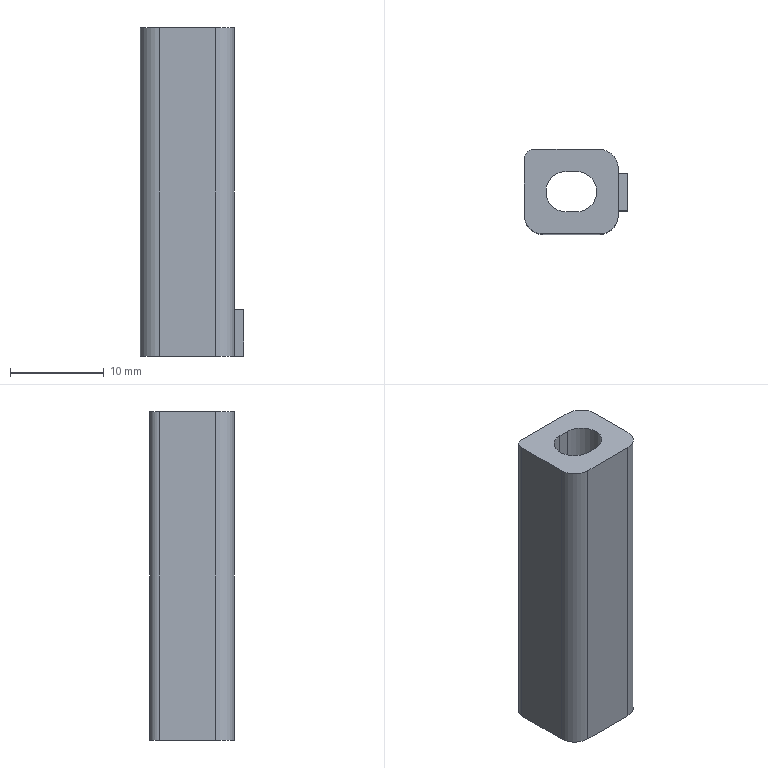Part | NX | features DIE-92 2 | 1 solid | 23 faces | box 11 x 9 x 35 mm | volume 2133 mm3 | plane 15 | cylinder 8 | commonest cylinder face diameters 4 x3 4.32 x2 5.32 x2 2 x1
STEP:
#1=CARTESIAN_POINT('',(4117.786,-841.782,823.716));
#2=VERTEX_POINT('',#1);
#3=CARTESIAN_POINT('',(4117.786,-836.462,823.716));
#4=VERTEX_POINT('',#3);
#5=CARTESIAN_POINT('',(4117.786,-839.122,823.716));
#6=DIRECTION('',(0.,0.,-1.));
#7=DIRECTION('',(-1.,0.,0.));
#8=AXIS2_PLACEMENT_3D('',#5,#6,#7);
#9=CIRCLE('',#8,2.66);
#10=EDGE_CURVE('',#2,#4,#9,.F.);
#11=ORIENTED_EDGE('',*,*,#10,.F.);
#12=CARTESIAN_POINT('',(4117.786,-841.782,853.716));
#13=VERTEX_POINT('',#12);
#14=CARTESIAN_POINT('',(4117.786,-841.782,862.216));
#15=DIRECTION('',(0.,0.,-1.));
#16=VECTOR('',#15,1000.);
#17=LINE('',#14,#16);
#18=EDGE_CURVE('',#2,#13,#17,.F.);
#19=ORIENTED_EDGE('',*,*,#18,.T.);
#20=CARTESIAN_POINT('',(4117.786,-836.462,853.716));
#21=VERTEX_POINT('',#20);
#22=CARTESIAN_POINT('',(4117.786,-839.122,853.716));
#23=DIRECTION('',(0.,0.,1.));
#24=DIRECTION('',(1.,0.,0.));
#25=AXIS2_PLACEMENT_3D('',#22,#23,#24);
#26=CIRCLE('',#25,2.66);
#27=EDGE_CURVE('',#21,#13,#26,.F.);
#28=ORIENTED_EDGE('',*,*,#27,.F.);
#29=CARTESIAN_POINT('',(4117.786,-836.462,862.216));
#30=DIRECTION('',(0.,0.,-1.));
#31=VECTOR('',#30,1000.);
#32=LINE('',#29,#31);
#33=EDGE_CURVE('',#21,#4,#32,.T.);
#34=ORIENTED_EDGE('',*,*,#33,.T.);
#35=EDGE_LOOP('',(#11,#19,#28,#34));
#36=FACE_BOUND('',#35,.T.);
#37=CARTESIAN_POINT('',(4117.786,-839.122,862.216));
#38=DIRECTION('',(0.,0.,-1.));
#39=DIRECTION('',(-1.,0.,0.));
#40=AXIS2_PLACEMENT_3D('',#37,#38,#39);
#41=CYLINDRICAL_SURFACE('',#40,2.66);
#42=ADVANCED_FACE('',(#36),#41,.F.);
#43=ORIENTED_EDGE('',*,*,#18,.F.);
#44=CARTESIAN_POINT('',(4116.686,-841.782,823.716));
#45=VERTEX_POINT('',#44);
#46=CARTESIAN_POINT('',(4123.586,-841.782,823.716));
#47=DIRECTION('',(1.,0.,0.));
#48=VECTOR('',#47,1000.);
#49=LINE('',#46,#48);
#50=EDGE_CURVE('',#45,#2,#49,.T.);
#51=ORIENTED_EDGE('',*,*,#50,.F.);
#52=CARTESIAN_POINT('',(4116.686,-841.782,853.716));
#53=VERTEX_POINT('',#52);
#54=CARTESIAN_POINT('',(4116.686,-841.782,862.216));
#55=DIRECTION('',(0.,0.,-1.));
#56=VECTOR('',#55,1000.);
#57=LINE('',#54,#56);
#58=EDGE_CURVE('',#53,#45,#57,.T.);
#59=ORIENTED_EDGE('',*,*,#58,.F.);
#60=CARTESIAN_POINT('',(4116.576,-841.782,853.716));
#61=DIRECTION('',(1.,0.,0.));
#62=VECTOR('',#61,1000.);
#63=LINE('',#60,#62);
#64=EDGE_CURVE('',#53,#13,#63,.T.);
#65=ORIENTED_EDGE('',*,*,#64,.T.);
#66=EDGE_LOOP('',(#43,#51,#59,#65));
#67=FACE_BOUND('',#66,.T.);
#68=CARTESIAN_POINT('',(4116.576,-841.782,870.016));
#69=DIRECTION('',(0.,1.,0.));
#70=DIRECTION('',(1.,0.,0.));
#71=AXIS2_PLACEMENT_3D('',#68,#69,#70);
#72=PLANE('',#71);
#73=ADVANCED_FACE('',(#67),#72,.T.);
#74=CARTESIAN_POINT('',(4116.686,-836.462,823.716));
#75=VERTEX_POINT('',#74);
#76=CARTESIAN_POINT('',(4116.686,-839.122,823.716));
#77=DIRECTION('',(0.,0.,-1.));
#78=DIRECTION('',(-1.,0.,0.));
#79=AXIS2_PLACEMENT_3D('',#76,#77,#78);
#80=CIRCLE('',#79,2.66);
#81=EDGE_CURVE('',#75,#45,#80,.F.);
#82=ORIENTED_EDGE('',*,*,#81,.F.);
#83=CARTESIAN_POINT('',(4116.686,-836.462,853.716));
#84=VERTEX_POINT('',#83);
#85=CARTESIAN_POINT('',(4116.686,-836.462,862.216));
#86=DIRECTION('',(0.,0.,-1.));
#87=VECTOR('',#86,1000.);
#88=LINE('',#85,#87);
#89=EDGE_CURVE('',#75,#84,#88,.F.);
#90=ORIENTED_EDGE('',*,*,#89,.T.);
#91=CARTESIAN_POINT('',(4116.686,-839.122,853.716));
#92=DIRECTION('',(0.,0.,1.));
#93=DIRECTION('',(1.,0.,0.));
#94=AXIS2_PLACEMENT_3D('',#91,#92,#93);
#95=CIRCLE('',#94,2.66);
#96=EDGE_CURVE('',#53,#84,#95,.F.);
#97=ORIENTED_EDGE('',*,*,#96,.F.);
#98=ORIENTED_EDGE('',*,*,#58,.T.);
#99=EDGE_LOOP('',(#82,#90,#97,#98));
#100=FACE_BOUND('',#99,.T.);
#101=CARTESIAN_POINT('',(4116.686,-839.122,862.216));
#102=DIRECTION('',(0.,0.,-1.));
#103=DIRECTION('',(1.,0.,0.));
#104=AXIS2_PLACEMENT_3D('',#101,#102,#103);
#105=CYLINDRICAL_SURFACE('',#104,2.66);
#106=ADVANCED_FACE('',(#100),#105,.F.);
#107=ORIENTED_EDGE('',*,*,#89,.F.);
#108=CARTESIAN_POINT('',(4117.896,-836.462,823.716));
#109=DIRECTION('',(1.,0.,0.));
#110=VECTOR('',#109,1000.);
#111=LINE('',#108,#110);
#112=EDGE_CURVE('',#75,#4,#111,.T.);
#113=ORIENTED_EDGE('',*,*,#112,.T.);
#114=ORIENTED_EDGE('',*,*,#33,.F.);
#115=CARTESIAN_POINT('',(4117.896,-836.462,853.716));
#116=DIRECTION('',(-1.,0.,0.));
#117=VECTOR('',#116,1000.);
#118=LINE('',#115,#117);
#119=EDGE_CURVE('',#21,#84,#118,.T.);
#120=ORIENTED_EDGE('',*,*,#119,.T.);
#121=EDGE_LOOP('',(#107,#113,#114,#120));
#122=FACE_BOUND('',#121,.T.);
#123=CARTESIAN_POINT('',(4117.896,-836.462,870.016));
#124=DIRECTION('',(0.,-1.,0.));
#125=DIRECTION('',(-1.,0.,0.));
#126=AXIS2_PLACEMENT_3D('',#123,#124,#125);
#127=PLANE('',#126);
#128=ADVANCED_FACE('',(#122),#127,.T.);
#129=CARTESIAN_POINT('',(4122.236,-837.122,823.716));
#130=VERTEX_POINT('',#129);
#131=CARTESIAN_POINT('',(4122.236,-836.622,823.716));
#132=VERTEX_POINT('',#131);
#133=CARTESIAN_POINT('',(4122.236,-839.122,823.716));
#134=DIRECTION('',(0.,1.,0.));
#135=VECTOR('',#134,1000.);
#136=LINE('',#133,#135);
#137=EDGE_CURVE('',#130,#132,#136,.T.);
#138=ORIENTED_EDGE('',*,*,#137,.F.);
#139=CARTESIAN_POINT('',(4123.236,-837.122,823.716));
#140=VERTEX_POINT('',#139);
#141=CARTESIAN_POINT('',(0.,-837.122,823.716));
#142=DIRECTION('',(1.,0.,0.));
#143=VECTOR('',#142,1000.);
#144=LINE('',#141,#143);
#145=EDGE_CURVE('',#130,#140,#144,.T.);
#146=ORIENTED_EDGE('',*,*,#145,.T.);
#147=CARTESIAN_POINT('',(4123.236,-841.122,823.716));
#148=VERTEX_POINT('',#147);
#149=CARTESIAN_POINT('',(4123.236,-836.622,823.716));
#150=DIRECTION('',(0.,-1.,0.));
#151=VECTOR('',#150,1000.);
#152=LINE('',#149,#151);
#153=EDGE_CURVE('',#140,#148,#152,.T.);
#154=ORIENTED_EDGE('',*,*,#153,.T.);
#155=CARTESIAN_POINT('',(4122.236,-841.122,823.716));
#156=VERTEX_POINT('',#155);
#157=CARTESIAN_POINT('',(0.,-841.122,823.716));
#158=DIRECTION('',(-1.,0.,0.));
#159=VECTOR('',#158,1000.);
#160=LINE('',#157,#159);
#161=EDGE_CURVE('',#148,#156,#160,.T.);
#162=ORIENTED_EDGE('',*,*,#161,.T.);
#163=CARTESIAN_POINT('',(4122.236,-841.622,823.716));
#164=VERTEX_POINT('',#163);
#165=CARTESIAN_POINT('',(4122.236,-839.122,823.716));
#166=DIRECTION('',(0.,1.,0.));
#167=VECTOR('',#166,1000.);
#168=LINE('',#165,#167);
#169=EDGE_CURVE('',#164,#156,#168,.T.);
#170=ORIENTED_EDGE('',*,*,#169,.F.);
#171=CARTESIAN_POINT('',(4120.236,-843.622,823.716));
#172=VERTEX_POINT('',#171);
#173=CARTESIAN_POINT('',(4120.236,-841.622,823.716));
#174=DIRECTION('',(0.,0.,-1.));
#175=DIRECTION('',(-1.,0.,0.));
#176=AXIS2_PLACEMENT_3D('',#173,#174,#175);
#177=CIRCLE('',#176,2.);
#178=EDGE_CURVE('',#164,#172,#177,.T.);
#179=ORIENTED_EDGE('',*,*,#178,.T.);
#180=CARTESIAN_POINT('',(4114.236,-843.622,823.716));
#181=VERTEX_POINT('',#180);
#182=CARTESIAN_POINT('',(4117.236,-843.622,823.716));
#183=DIRECTION('',(1.,0.,0.));
#184=VECTOR('',#183,1000.);
#185=LINE('',#182,#184);
#186=EDGE_CURVE('',#181,#172,#185,.T.);
#187=ORIENTED_EDGE('',*,*,#186,.F.);
#188=CARTESIAN_POINT('',(4112.236,-841.622,823.716));
#189=VERTEX_POINT('',#188);
#190=CARTESIAN_POINT('',(4114.236,-841.622,823.716));
#191=DIRECTION('',(0.,0.,-1.));
#192=DIRECTION('',(-1.,0.,0.));
#193=AXIS2_PLACEMENT_3D('',#190,#191,#192);
#194=CIRCLE('',#193,2.);
#195=EDGE_CURVE('',#181,#189,#194,.T.);
#196=ORIENTED_EDGE('',*,*,#195,.T.);
#197=CARTESIAN_POINT('',(4112.236,-835.622,823.716));
#198=VERTEX_POINT('',#197);
#199=CARTESIAN_POINT('',(4112.236,-839.122,823.716));
#200=DIRECTION('',(0.,-1.,0.));
#201=VECTOR('',#200,1000.);
#202=LINE('',#199,#201);
#203=EDGE_CURVE('',#198,#189,#202,.T.);
#204=ORIENTED_EDGE('',*,*,#203,.F.);
#205=CARTESIAN_POINT('',(4113.236,-834.622,823.716));
#206=VERTEX_POINT('',#205);
#207=CARTESIAN_POINT('',(4113.236,-835.622,823.716));
#208=DIRECTION('',(0.,0.,-1.));
#209=DIRECTION('',(-1.,0.,0.));
#210=AXIS2_PLACEMENT_3D('',#207,#208,#209);
#211=CIRCLE('',#210,1.);
#212=EDGE_CURVE('',#206,#198,#211,.F.);
#213=ORIENTED_EDGE('',*,*,#212,.F.);
#214=CARTESIAN_POINT('',(4120.236,-834.622,823.716));
#215=VERTEX_POINT('',#214);
#216=CARTESIAN_POINT('',(4117.236,-834.622,823.716));
#217=DIRECTION('',(-1.,0.,0.));
#218=VECTOR('',#217,1000.);
#219=LINE('',#216,#218);
#220=EDGE_CURVE('',#206,#215,#219,.F.);
#221=ORIENTED_EDGE('',*,*,#220,.T.);
#222=CARTESIAN_POINT('',(4120.236,-836.622,823.716));
#223=DIRECTION('',(0.,0.,-1.));
#224=DIRECTION('',(-1.,0.,0.));
#225=AXIS2_PLACEMENT_3D('',#222,#223,#224);
#226=CIRCLE('',#225,2.);
#227=EDGE_CURVE('',#215,#132,#226,.T.);
#228=ORIENTED_EDGE('',*,*,#227,.T.);
#229=EDGE_LOOP('',(#138,#146,#154,#162,#170,#179,#187,#196,#204,#213,#221,#228));
#230=FACE_BOUND('',#229,.T.);
#231=ORIENTED_EDGE('',*,*,#112,.F.);
#232=ORIENTED_EDGE('',*,*,#81,.T.);
#233=ORIENTED_EDGE('',*,*,#50,.T.);
#234=ORIENTED_EDGE('',*,*,#10,.T.);
#235=EDGE_LOOP('',(#231,#232,#233,#234));
#236=FACE_BOUND('',#235,.T.);
#237=CARTESIAN_POINT('',(4123.586,-858.122,823.716));
#238=DIRECTION('',(0.,0.,-1.));
#239=DIRECTION('',(-1.,0.,0.));
#240=AXIS2_PLACEMENT_3D('',#237,#238,#239);
#241=PLANE('',#240);
#242=ADVANCED_FACE('',(#230,#236),#241,.T.);
#243=CARTESIAN_POINT('',(4117.786,-841.282,853.716));
#244=VERTEX_POINT('',#243);
#245=CARTESIAN_POINT('',(4116.686,-841.282,853.716));
#246=VERTEX_POINT('',#245);
#247=CARTESIAN_POINT('',(4116.576,-841.282,853.716));
#248=DIRECTION('',(1.,0.,0.));
#249=VECTOR('',#248,1000.);
#250=LINE('',#247,#249);
#251=EDGE_CURVE('',#244,#246,#250,.F.);
#252=ORIENTED_EDGE('',*,*,#251,.F.);
#253=CARTESIAN_POINT('',(4117.786,-836.962,853.716));
#254=VERTEX_POINT('',#253);
#255=CARTESIAN_POINT('',(4117.786,-839.122,853.716));
#256=DIRECTION('',(0.,0.,1.));
#257=DIRECTION('',(1.,0.,0.));
#258=AXIS2_PLACEMENT_3D('',#255,#256,#257);
#259=CIRCLE('',#258,2.16);
#260=EDGE_CURVE('',#244,#254,#259,.T.);
#261=ORIENTED_EDGE('',*,*,#260,.T.);
#262=CARTESIAN_POINT('',(4116.686,-836.962,853.716));
#263=VERTEX_POINT('',#262);
#264=CARTESIAN_POINT('',(4117.896,-836.962,853.716));
#265=DIRECTION('',(-1.,0.,0.));
#266=VECTOR('',#265,1000.);
#267=LINE('',#264,#266);
#268=EDGE_CURVE('',#263,#254,#267,.F.);
#269=ORIENTED_EDGE('',*,*,#268,.F.);
#270=CARTESIAN_POINT('',(4116.686,-839.122,853.716));
#271=DIRECTION('',(0.,0.,1.));
#272=DIRECTION('',(1.,0.,0.));
#273=AXIS2_PLACEMENT_3D('',#270,#271,#272);
#274=CIRCLE('',#273,2.16);
#275=EDGE_CURVE('',#263,#246,#274,.T.);
#276=ORIENTED_EDGE('',*,*,#275,.T.);
#277=EDGE_LOOP('',(#252,#261,#269,#276));
#278=FACE_BOUND('',#277,.T.);
#279=ORIENTED_EDGE('',*,*,#64,.F.);
#280=ORIENTED_EDGE('',*,*,#96,.T.);
#281=ORIENTED_EDGE('',*,*,#119,.F.);
#282=ORIENTED_EDGE('',*,*,#27,.T.);
#283=EDGE_LOOP('',(#279,#280,#281,#282));
#284=FACE_BOUND('',#283,.T.);
#285=CARTESIAN_POINT('',(4079.736,-858.122,853.716));
#286=DIRECTION('',(0.,0.,1.));
#287=DIRECTION('',(1.,0.,0.));
#288=AXIS2_PLACEMENT_3D('',#285,#286,#287);
#289=PLANE('',#288);
#290=ADVANCED_FACE('',(#278,#284),#289,.F.);
#291=ORIENTED_EDGE('',*,*,#251,.T.);
#292=CARTESIAN_POINT('',(4116.686,-841.282,858.716));
#293=VERTEX_POINT('',#292);
#294=CARTESIAN_POINT('',(4116.686,-841.282,862.216));
#295=DIRECTION('',(0.,0.,-1.));
#296=VECTOR('',#295,1000.);
#297=LINE('',#294,#296);
#298=EDGE_CURVE('',#293,#246,#297,.T.);
#299=ORIENTED_EDGE('',*,*,#298,.F.);
#300=CARTESIAN_POINT('',(4117.786,-841.282,858.716));
#301=VERTEX_POINT('',#300);
#302=CARTESIAN_POINT('',(4123.586,-841.282,858.716));
#303=DIRECTION('',(-1.,0.,0.));
#304=VECTOR('',#303,1000.);
#305=LINE('',#302,#304);
#306=EDGE_CURVE('',#301,#293,#305,.T.);
#307=ORIENTED_EDGE('',*,*,#306,.F.);
#308=CARTESIAN_POINT('',(4117.786,-841.282,862.216));
#309=DIRECTION('',(0.,0.,-1.));
#310=VECTOR('',#309,1000.);
#311=LINE('',#308,#310);
#312=EDGE_CURVE('',#244,#301,#311,.F.);
#313=ORIENTED_EDGE('',*,*,#312,.F.);
#314=EDGE_LOOP('',(#291,#299,#307,#313));
#315=FACE_BOUND('',#314,.T.);
#316=CARTESIAN_POINT('',(4116.576,-841.282,870.016));
#317=DIRECTION('',(0.,1.,0.));
#318=DIRECTION('',(1.,0.,0.));
#319=AXIS2_PLACEMENT_3D('',#316,#317,#318);
#320=PLANE('',#319);
#321=ADVANCED_FACE('',(#315),#320,.T.);
#322=CARTESIAN_POINT('',(4117.786,-836.962,858.716));
#323=VERTEX_POINT('',#322);
#324=CARTESIAN_POINT('',(4117.786,-836.962,862.216));
#325=DIRECTION('',(0.,0.,-1.));
#326=VECTOR('',#325,1000.);
#327=LINE('',#324,#326);
#328=EDGE_CURVE('',#323,#254,#327,.T.);
#329=ORIENTED_EDGE('',*,*,#328,.T.);
#330=ORIENTED_EDGE('',*,*,#260,.F.);
#331=ORIENTED_EDGE('',*,*,#312,.T.);
#332=CARTESIAN_POINT('',(4117.786,-839.122,858.716));
#333=DIRECTION('',(0.,0.,1.));
#334=DIRECTION('',(1.,0.,0.));
#335=AXIS2_PLACEMENT_3D('',#332,#333,#334);
#336=CIRCLE('',#335,2.16);
#337=EDGE_CURVE('',#301,#323,#336,.T.);
#338=ORIENTED_EDGE('',*,*,#337,.T.);
#339=EDGE_LOOP('',(#329,#330,#331,#338));
#340=FACE_BOUND('',#339,.T.);
#341=CARTESIAN_POINT('',(4117.786,-839.122,862.216));
#342=DIRECTION('',(0.,0.,-1.));
#343=DIRECTION('',(-1.,0.,0.));
#344=AXIS2_PLACEMENT_3D('',#341,#342,#343);
#345=CYLINDRICAL_SURFACE('',#344,2.16);
#346=ADVANCED_FACE('',(#340),#345,.F.);
#347=ORIENTED_EDGE('',*,*,#268,.T.);
#348=ORIENTED_EDGE('',*,*,#328,.F.);
#349=CARTESIAN_POINT('',(4116.686,-836.962,858.716));
#350=VERTEX_POINT('',#349);
#351=CARTESIAN_POINT('',(4123.586,-836.962,858.716));
#352=DIRECTION('',(1.,0.,0.));
#353=VECTOR('',#352,1000.);
#354=LINE('',#351,#353);
#355=EDGE_CURVE('',#350,#323,#354,.T.);
#356=ORIENTED_EDGE('',*,*,#355,.F.);
#357=CARTESIAN_POINT('',(4116.686,-836.962,862.216));
#358=DIRECTION('',(0.,0.,-1.));
#359=VECTOR('',#358,1000.);
#360=LINE('',#357,#359);
#361=EDGE_CURVE('',#263,#350,#360,.F.);
#362=ORIENTED_EDGE('',*,*,#361,.F.);
#363=EDGE_LOOP('',(#347,#348,#356,#362));
#364=FACE_BOUND('',#363,.T.);
#365=CARTESIAN_POINT('',(4117.896,-836.962,870.016));
#366=DIRECTION('',(0.,-1.,0.));
#367=DIRECTION('',(-1.,0.,0.));
#368=AXIS2_PLACEMENT_3D('',#365,#366,#367);
#369=PLANE('',#368);
#370=ADVANCED_FACE('',(#364),#369,.T.);
#371=ORIENTED_EDGE('',*,*,#298,.T.);
#372=ORIENTED_EDGE('',*,*,#275,.F.);
#373=ORIENTED_EDGE('',*,*,#361,.T.);
#374=CARTESIAN_POINT('',(4116.686,-839.122,858.716));
#375=DIRECTION('',(0.,0.,1.));
#376=DIRECTION('',(1.,0.,0.));
#377=AXIS2_PLACEMENT_3D('',#374,#375,#376);
#378=CIRCLE('',#377,2.16);
#379=EDGE_CURVE('',#350,#293,#378,.T.);
#380=ORIENTED_EDGE('',*,*,#379,.T.);
#381=EDGE_LOOP('',(#371,#372,#373,#380));
#382=FACE_BOUND('',#381,.T.);
#383=CARTESIAN_POINT('',(4116.686,-839.122,862.216));
#384=DIRECTION('',(0.,0.,-1.));
#385=DIRECTION('',(1.,0.,0.));
#386=AXIS2_PLACEMENT_3D('',#383,#384,#385);
#387=CYLINDRICAL_SURFACE('',#386,2.16);
#388=ADVANCED_FACE('',(#382),#387,.F.);
#389=ORIENTED_EDGE('',*,*,#379,.F.);
#390=ORIENTED_EDGE('',*,*,#355,.T.);
#391=ORIENTED_EDGE('',*,*,#337,.F.);
#392=ORIENTED_EDGE('',*,*,#306,.T.);
#393=EDGE_LOOP('',(#389,#390,#391,#392));
#394=FACE_BOUND('',#393,.T.);
#395=CARTESIAN_POINT('',(4112.236,-841.622,858.716));
#396=VERTEX_POINT('',#395);
#397=CARTESIAN_POINT('',(4112.236,-835.622,858.716));
#398=VERTEX_POINT('',#397);
#399=CARTESIAN_POINT('',(4112.236,-839.122,858.716));
#400=DIRECTION('',(0.,1.,0.));
#401=VECTOR('',#400,1000.);
#402=LINE('',#399,#401);
#403=EDGE_CURVE('',#396,#398,#402,.T.);
#404=ORIENTED_EDGE('',*,*,#403,.F.);
#405=CARTESIAN_POINT('',(4114.236,-843.622,858.716));
#406=VERTEX_POINT('',#405);
#407=CARTESIAN_POINT('',(4114.236,-841.622,858.716));
#408=DIRECTION('',(0.,0.,1.));
#409=DIRECTION('',(1.,0.,0.));
#410=AXIS2_PLACEMENT_3D('',#407,#408,#409);
#411=CIRCLE('',#410,2.);
#412=EDGE_CURVE('',#396,#406,#411,.T.);
#413=ORIENTED_EDGE('',*,*,#412,.T.);
#414=CARTESIAN_POINT('',(4120.236,-843.622,858.716));
#415=VERTEX_POINT('',#414);
#416=CARTESIAN_POINT('',(4117.236,-843.622,858.716));
#417=DIRECTION('',(-1.,0.,0.));
#418=VECTOR('',#417,1000.);
#419=LINE('',#416,#418);
#420=EDGE_CURVE('',#406,#415,#419,.F.);
#421=ORIENTED_EDGE('',*,*,#420,.T.);
#422=CARTESIAN_POINT('',(4122.236,-841.622,858.716));
#423=VERTEX_POINT('',#422);
#424=CARTESIAN_POINT('',(4120.236,-841.622,858.716));
#425=DIRECTION('',(0.,0.,1.));
#426=DIRECTION('',(1.,0.,0.));
#427=AXIS2_PLACEMENT_3D('',#424,#425,#426);
#428=CIRCLE('',#427,2.);
#429=EDGE_CURVE('',#423,#415,#428,.F.);
#430=ORIENTED_EDGE('',*,*,#429,.F.);
#431=CARTESIAN_POINT('',(4122.236,-836.622,858.716));
#432=VERTEX_POINT('',#431);
#433=CARTESIAN_POINT('',(4122.236,-839.122,858.716));
#434=DIRECTION('',(0.,-1.,0.));
#435=VECTOR('',#434,1000.);
#436=LINE('',#433,#435);
#437=EDGE_CURVE('',#423,#432,#436,.F.);
#438=ORIENTED_EDGE('',*,*,#437,.T.);
#439=CARTESIAN_POINT('',(4120.236,-834.622,858.716));
#440=VERTEX_POINT('',#439);
#441=CARTESIAN_POINT('',(4120.236,-836.622,858.716));
#442=DIRECTION('',(0.,0.,1.));
#443=DIRECTION('',(1.,0.,0.));
#444=AXIS2_PLACEMENT_3D('',#441,#442,#443);
#445=CIRCLE('',#444,2.);
#446=EDGE_CURVE('',#440,#432,#445,.F.);
#447=ORIENTED_EDGE('',*,*,#446,.F.);
#448=CARTESIAN_POINT('',(4113.236,-834.622,858.716));
#449=VERTEX_POINT('',#448);
#450=CARTESIAN_POINT('',(4117.236,-834.622,858.716));
#451=DIRECTION('',(1.,0.,0.));
#452=VECTOR('',#451,1000.);
#453=LINE('',#450,#452);
#454=EDGE_CURVE('',#449,#440,#453,.T.);
#455=ORIENTED_EDGE('',*,*,#454,.F.);
#456=CARTESIAN_POINT('',(4113.236,-835.622,858.716));
#457=DIRECTION('',(0.,0.,1.));
#458=DIRECTION('',(1.,0.,0.));
#459=AXIS2_PLACEMENT_3D('',#456,#457,#458);
#460=CIRCLE('',#459,1.);
#461=EDGE_CURVE('',#449,#398,#460,.T.);
#462=ORIENTED_EDGE('',*,*,#461,.T.);
#463=EDGE_LOOP('',(#404,#413,#421,#430,#438,#447,#455,#462));
#464=FACE_BOUND('',#463,.T.);
#465=CARTESIAN_POINT('',(4123.586,-858.122,858.716));
#466=DIRECTION('',(0.,0.,1.));
#467=DIRECTION('',(-1.,0.,0.));
#468=AXIS2_PLACEMENT_3D('',#465,#466,#467);
#469=PLANE('',#468);
#470=ADVANCED_FACE('',(#394,#464),#469,.T.);
#471=ORIENTED_EDGE('',*,*,#212,.T.);
#472=CARTESIAN_POINT('',(4112.236,-835.622,823.716));
#473=DIRECTION('',(0.,0.,1.));
#474=VECTOR('',#473,1000.);
#475=LINE('',#472,#474);
#476=EDGE_CURVE('',#398,#198,#475,.F.);
#477=ORIENTED_EDGE('',*,*,#476,.F.);
#478=ORIENTED_EDGE('',*,*,#461,.F.);
#479=CARTESIAN_POINT('',(4113.236,-834.622,823.716));
#480=DIRECTION('',(0.,0.,1.));
#481=VECTOR('',#480,1000.);
#482=LINE('',#479,#481);
#483=EDGE_CURVE('',#206,#449,#482,.T.);
#484=ORIENTED_EDGE('',*,*,#483,.F.);
#485=EDGE_LOOP('',(#471,#477,#478,#484));
#486=FACE_BOUND('',#485,.T.);
#487=CARTESIAN_POINT('',(4113.236,-835.622,823.716));
#488=DIRECTION('',(0.,0.,1.));
#489=DIRECTION('',(1.,0.,0.));
#490=AXIS2_PLACEMENT_3D('',#487,#488,#489);
#491=CYLINDRICAL_SURFACE('',#490,1.);
#492=ADVANCED_FACE('',(#486),#491,.T.);
#493=ORIENTED_EDGE('',*,*,#195,.F.);
#494=CARTESIAN_POINT('',(4114.236,-843.622,823.716));
#495=DIRECTION('',(0.,0.,1.));
#496=VECTOR('',#495,1000.);
#497=LINE('',#494,#496);
#498=EDGE_CURVE('',#406,#181,#497,.F.);
#499=ORIENTED_EDGE('',*,*,#498,.F.);
#500=ORIENTED_EDGE('',*,*,#412,.F.);
#501=CARTESIAN_POINT('',(4112.236,-841.622,823.716));
#502=DIRECTION('',(0.,0.,1.));
#503=VECTOR('',#502,1000.);
#504=LINE('',#501,#503);
#505=EDGE_CURVE('',#189,#396,#504,.T.);
#506=ORIENTED_EDGE('',*,*,#505,.F.);
#507=EDGE_LOOP('',(#493,#499,#500,#506));
#508=FACE_BOUND('',#507,.T.);
#509=CARTESIAN_POINT('',(4114.236,-841.622,823.716));
#510=DIRECTION('',(0.,0.,1.));
#511=DIRECTION('',(1.,0.,0.));
#512=AXIS2_PLACEMENT_3D('',#509,#510,#511);
#513=CYLINDRICAL_SURFACE('',#512,2.);
#514=ADVANCED_FACE('',(#508),#513,.T.);
#515=ORIENTED_EDGE('',*,*,#178,.F.);
#516=CARTESIAN_POINT('',(4122.236,-841.622,823.716));
#517=DIRECTION('',(0.,0.,1.));
#518=VECTOR('',#517,1000.);
#519=LINE('',#516,#518);
#520=EDGE_CURVE('',#423,#164,#519,.F.);
#521=ORIENTED_EDGE('',*,*,#520,.F.);
#522=ORIENTED_EDGE('',*,*,#429,.T.);
#523=CARTESIAN_POINT('',(4120.236,-843.622,823.716));
#524=DIRECTION('',(0.,0.,1.));
#525=VECTOR('',#524,1000.);
#526=LINE('',#523,#525);
#527=EDGE_CURVE('',#172,#415,#526,.T.);
#528=ORIENTED_EDGE('',*,*,#527,.F.);
#529=EDGE_LOOP('',(#515,#521,#522,#528));
#530=FACE_BOUND('',#529,.T.);
#531=CARTESIAN_POINT('',(4120.236,-841.622,823.716));
#532=DIRECTION('',(0.,0.,1.));
#533=DIRECTION('',(1.,0.,0.));
#534=AXIS2_PLACEMENT_3D('',#531,#532,#533);
#535=CYLINDRICAL_SURFACE('',#534,2.);
#536=ADVANCED_FACE('',(#530),#535,.T.);
#537=ORIENTED_EDGE('',*,*,#227,.F.);
#538=CARTESIAN_POINT('',(4120.236,-834.622,823.716));
#539=DIRECTION('',(0.,0.,1.));
#540=VECTOR('',#539,1000.);
#541=LINE('',#538,#540);
#542=EDGE_CURVE('',#440,#215,#541,.F.);
#543=ORIENTED_EDGE('',*,*,#542,.F.);
#544=ORIENTED_EDGE('',*,*,#446,.T.);
#545=CARTESIAN_POINT('',(4122.236,-836.622,823.716));
#546=DIRECTION('',(0.,0.,1.));
#547=VECTOR('',#546,1000.);
#548=LINE('',#545,#547);
#549=EDGE_CURVE('',#132,#432,#548,.T.);
#550=ORIENTED_EDGE('',*,*,#549,.F.);
#551=EDGE_LOOP('',(#537,#543,#544,#550));
#552=FACE_BOUND('',#551,.T.);
#553=CARTESIAN_POINT('',(4120.236,-836.622,823.716));
#554=DIRECTION('',(0.,0.,1.));
#555=DIRECTION('',(1.,0.,0.));
#556=AXIS2_PLACEMENT_3D('',#553,#554,#555);
#557=CYLINDRICAL_SURFACE('',#556,2.);
#558=ADVANCED_FACE('',(#552),#557,.T.);
#559=CARTESIAN_POINT('',(4122.236,-841.122,828.716));
#560=VERTEX_POINT('',#559);
#561=CARTESIAN_POINT('',(4122.236,-841.122,823.716));
#562=DIRECTION('',(0.,0.,-1.));
#563=VECTOR('',#562,1000.);
#564=LINE('',#561,#563);
#565=EDGE_CURVE('',#560,#156,#564,.T.);
#566=ORIENTED_EDGE('',*,*,#565,.F.);
#567=CARTESIAN_POINT('',(4122.236,-837.122,828.716));
#568=VERTEX_POINT('',#567);
#569=CARTESIAN_POINT('',(4122.236,-839.122,828.716));
#570=DIRECTION('',(0.,1.,0.));
#571=VECTOR('',#570,1000.);
#572=LINE('',#569,#571);
#573=EDGE_CURVE('',#560,#568,#572,.T.);
#574=ORIENTED_EDGE('',*,*,#573,.T.);
#575=CARTESIAN_POINT('',(4122.236,-837.122,823.716));
#576=DIRECTION('',(0.,0.,1.));
#577=VECTOR('',#576,1000.);
#578=LINE('',#575,#577);
#579=EDGE_CURVE('',#130,#568,#578,.T.);
#580=ORIENTED_EDGE('',*,*,#579,.F.);
#581=ORIENTED_EDGE('',*,*,#137,.T.);
#582=ORIENTED_EDGE('',*,*,#549,.T.);
#583=ORIENTED_EDGE('',*,*,#437,.F.);
#584=ORIENTED_EDGE('',*,*,#520,.T.);
#585=ORIENTED_EDGE('',*,*,#169,.T.);
#586=EDGE_LOOP('',(#566,#574,#580,#581,#582,#583,#584,#585));
#587=FACE_BOUND('',#586,.T.);
#588=CARTESIAN_POINT('',(4122.236,-839.122,823.716));
#589=DIRECTION('',(1.,0.,0.));
#590=DIRECTION('',(0.,0.,-1.));
#591=AXIS2_PLACEMENT_3D('',#588,#589,#590);
#592=PLANE('',#591);
#593=ADVANCED_FACE('',(#587),#592,.T.);
#594=ORIENTED_EDGE('',*,*,#220,.F.);
#595=ORIENTED_EDGE('',*,*,#483,.T.);
#596=ORIENTED_EDGE('',*,*,#454,.T.);
#597=ORIENTED_EDGE('',*,*,#542,.T.);
#598=EDGE_LOOP('',(#594,#595,#596,#597));
#599=FACE_BOUND('',#598,.T.);
#600=CARTESIAN_POINT('',(4117.236,-834.622,823.716));
#601=DIRECTION('',(0.,1.,0.));
#602=DIRECTION('',(0.,0.,1.));
#603=AXIS2_PLACEMENT_3D('',#600,#601,#602);
#604=PLANE('',#603);
#605=ADVANCED_FACE('',(#599),#604,.T.);
#606=ORIENTED_EDGE('',*,*,#403,.T.);
#607=ORIENTED_EDGE('',*,*,#476,.T.);
#608=ORIENTED_EDGE('',*,*,#203,.T.);
#609=ORIENTED_EDGE('',*,*,#505,.T.);
#610=EDGE_LOOP('',(#606,#607,#608,#609));
#611=FACE_BOUND('',#610,.T.);
#612=CARTESIAN_POINT('',(4112.236,-839.122,823.716));
#613=DIRECTION('',(-1.,0.,0.));
#614=DIRECTION('',(0.,0.,1.));
#615=AXIS2_PLACEMENT_3D('',#612,#613,#614);
#616=PLANE('',#615);
#617=ADVANCED_FACE('',(#611),#616,.T.);
#618=ORIENTED_EDGE('',*,*,#186,.T.);
#619=ORIENTED_EDGE('',*,*,#527,.T.);
#620=ORIENTED_EDGE('',*,*,#420,.F.);
#621=ORIENTED_EDGE('',*,*,#498,.T.);
#622=EDGE_LOOP('',(#618,#619,#620,#621));
#623=FACE_BOUND('',#622,.T.);
#624=CARTESIAN_POINT('',(4117.236,-843.622,823.716));
#625=DIRECTION('',(0.,-1.,0.));
#626=DIRECTION('',(0.,0.,-1.));
#627=AXIS2_PLACEMENT_3D('',#624,#625,#626);
#628=PLANE('',#627);
#629=ADVANCED_FACE('',(#623),#628,.T.);
#630=CARTESIAN_POINT('',(4123.236,-841.122,828.716));
#631=VERTEX_POINT('',#630);
#632=CARTESIAN_POINT('',(0.,-841.122,828.716));
#633=DIRECTION('',(-1.,0.,0.));
#634=VECTOR('',#633,1000.);
#635=LINE('',#632,#634);
#636=EDGE_CURVE('',#631,#560,#635,.T.);
#637=ORIENTED_EDGE('',*,*,#636,.T.);
#638=ORIENTED_EDGE('',*,*,#565,.T.);
#639=ORIENTED_EDGE('',*,*,#161,.F.);
#640=CARTESIAN_POINT('',(4123.236,-841.122,828.716));
#641=DIRECTION('',(0.,0.,-1.));
#642=VECTOR('',#641,1000.);
#643=LINE('',#640,#642);
#644=EDGE_CURVE('',#631,#148,#643,.T.);
#645=ORIENTED_EDGE('',*,*,#644,.F.);
#646=EDGE_LOOP('',(#637,#638,#639,#645));
#647=FACE_BOUND('',#646,.T.);
#648=CARTESIAN_POINT('',(4123.236,-841.122,828.716));
#649=DIRECTION('',(0.,-1.,0.));
#650=DIRECTION('',(0.,0.,-1.));
#651=AXIS2_PLACEMENT_3D('',#648,#649,#650);
#652=PLANE('',#651);
#653=ADVANCED_FACE('',(#647),#652,.T.);
#654=ORIENTED_EDGE('',*,*,#145,.F.);
#655=ORIENTED_EDGE('',*,*,#579,.T.);
#656=CARTESIAN_POINT('',(4123.236,-837.122,828.716));
#657=VERTEX_POINT('',#656);
#658=CARTESIAN_POINT('',(0.,-837.122,828.716));
#659=DIRECTION('',(1.,0.,0.));
#660=VECTOR('',#659,1000.);
#661=LINE('',#658,#660);
#662=EDGE_CURVE('',#568,#657,#661,.T.);
#663=ORIENTED_EDGE('',*,*,#662,.T.);
#664=CARTESIAN_POINT('',(4123.236,-837.122,828.716));
#665=DIRECTION('',(0.,0.,-1.));
#666=VECTOR('',#665,1000.);
#667=LINE('',#664,#666);
#668=EDGE_CURVE('',#657,#140,#667,.T.);
#669=ORIENTED_EDGE('',*,*,#668,.T.);
#670=EDGE_LOOP('',(#654,#655,#663,#669));
#671=FACE_BOUND('',#670,.T.);
#672=CARTESIAN_POINT('',(4122.186,-837.122,828.716));
#673=DIRECTION('',(0.,1.,0.));
#674=DIRECTION('',(0.,0.,1.));
#675=AXIS2_PLACEMENT_3D('',#672,#673,#674);
#676=PLANE('',#675);
#677=ADVANCED_FACE('',(#671),#676,.T.);
#678=ORIENTED_EDGE('',*,*,#153,.F.);
#679=ORIENTED_EDGE('',*,*,#668,.F.);
#680=CARTESIAN_POINT('',(4123.236,0.,828.716));
#681=DIRECTION('',(0.,-1.,0.));
#682=VECTOR('',#681,1000.);
#683=LINE('',#680,#682);
#684=EDGE_CURVE('',#657,#631,#683,.T.);
#685=ORIENTED_EDGE('',*,*,#684,.T.);
#686=ORIENTED_EDGE('',*,*,#644,.T.);
#687=EDGE_LOOP('',(#678,#679,#685,#686));
#688=FACE_BOUND('',#687,.T.);
#689=CARTESIAN_POINT('',(4123.236,-836.622,828.716));
#690=DIRECTION('',(1.,0.,0.));
#691=DIRECTION('',(0.,0.,-1.));
#692=AXIS2_PLACEMENT_3D('',#689,#690,#691);
#693=PLANE('',#692);
#694=ADVANCED_FACE('',(#688),#693,.T.);
#695=ORIENTED_EDGE('',*,*,#573,.F.);
#696=ORIENTED_EDGE('',*,*,#636,.F.);
#697=ORIENTED_EDGE('',*,*,#684,.F.);
#698=ORIENTED_EDGE('',*,*,#662,.F.);
#699=EDGE_LOOP('',(#695,#696,#697,#698));
#700=FACE_BOUND('',#699,.T.);
#701=CARTESIAN_POINT('',(0.,0.,828.716));
#702=DIRECTION('',(0.,0.,-1.));
#703=DIRECTION('',(-1.,0.,0.));
#704=AXIS2_PLACEMENT_3D('',#701,#702,#703);
#705=PLANE('',#704);
#706=ADVANCED_FACE('',(#700),#705,.F.);
#707=CLOSED_SHELL('',(#42,#73,#106,#128,#242,#290,#321,#346,#370,#388,#470,#492,#514,#536,#558,#593,#605,#617,#629,#653,#677,#694,#706));
#708=MANIFOLD_SOLID_BREP('',#707);
#709=(LENGTH_UNIT()NAMED_UNIT(*)SI_UNIT(.MILLI.,.METRE.));
#710=UNCERTAINTY_MEASURE_WITH_UNIT(LENGTH_MEASURE(0.00001),#709,'','');
#711=(NAMED_UNIT(*)PLANE_ANGLE_UNIT()SI_UNIT($,.RADIAN.));
#712=(NAMED_UNIT(*)SI_UNIT($,.STERADIAN.)SOLID_ANGLE_UNIT());
#713=(GEOMETRIC_REPRESENTATION_CONTEXT(3)GLOBAL_UNCERTAINTY_ASSIGNED_CONTEXT((#710))GLOBAL_UNIT_ASSIGNED_CONTEXT((#709,#711,#712))REPRESENTATION_CONTEXT('',''));
#714=ADVANCED_BREP_SHAPE_REPRESENTATION('',(#708),#713);